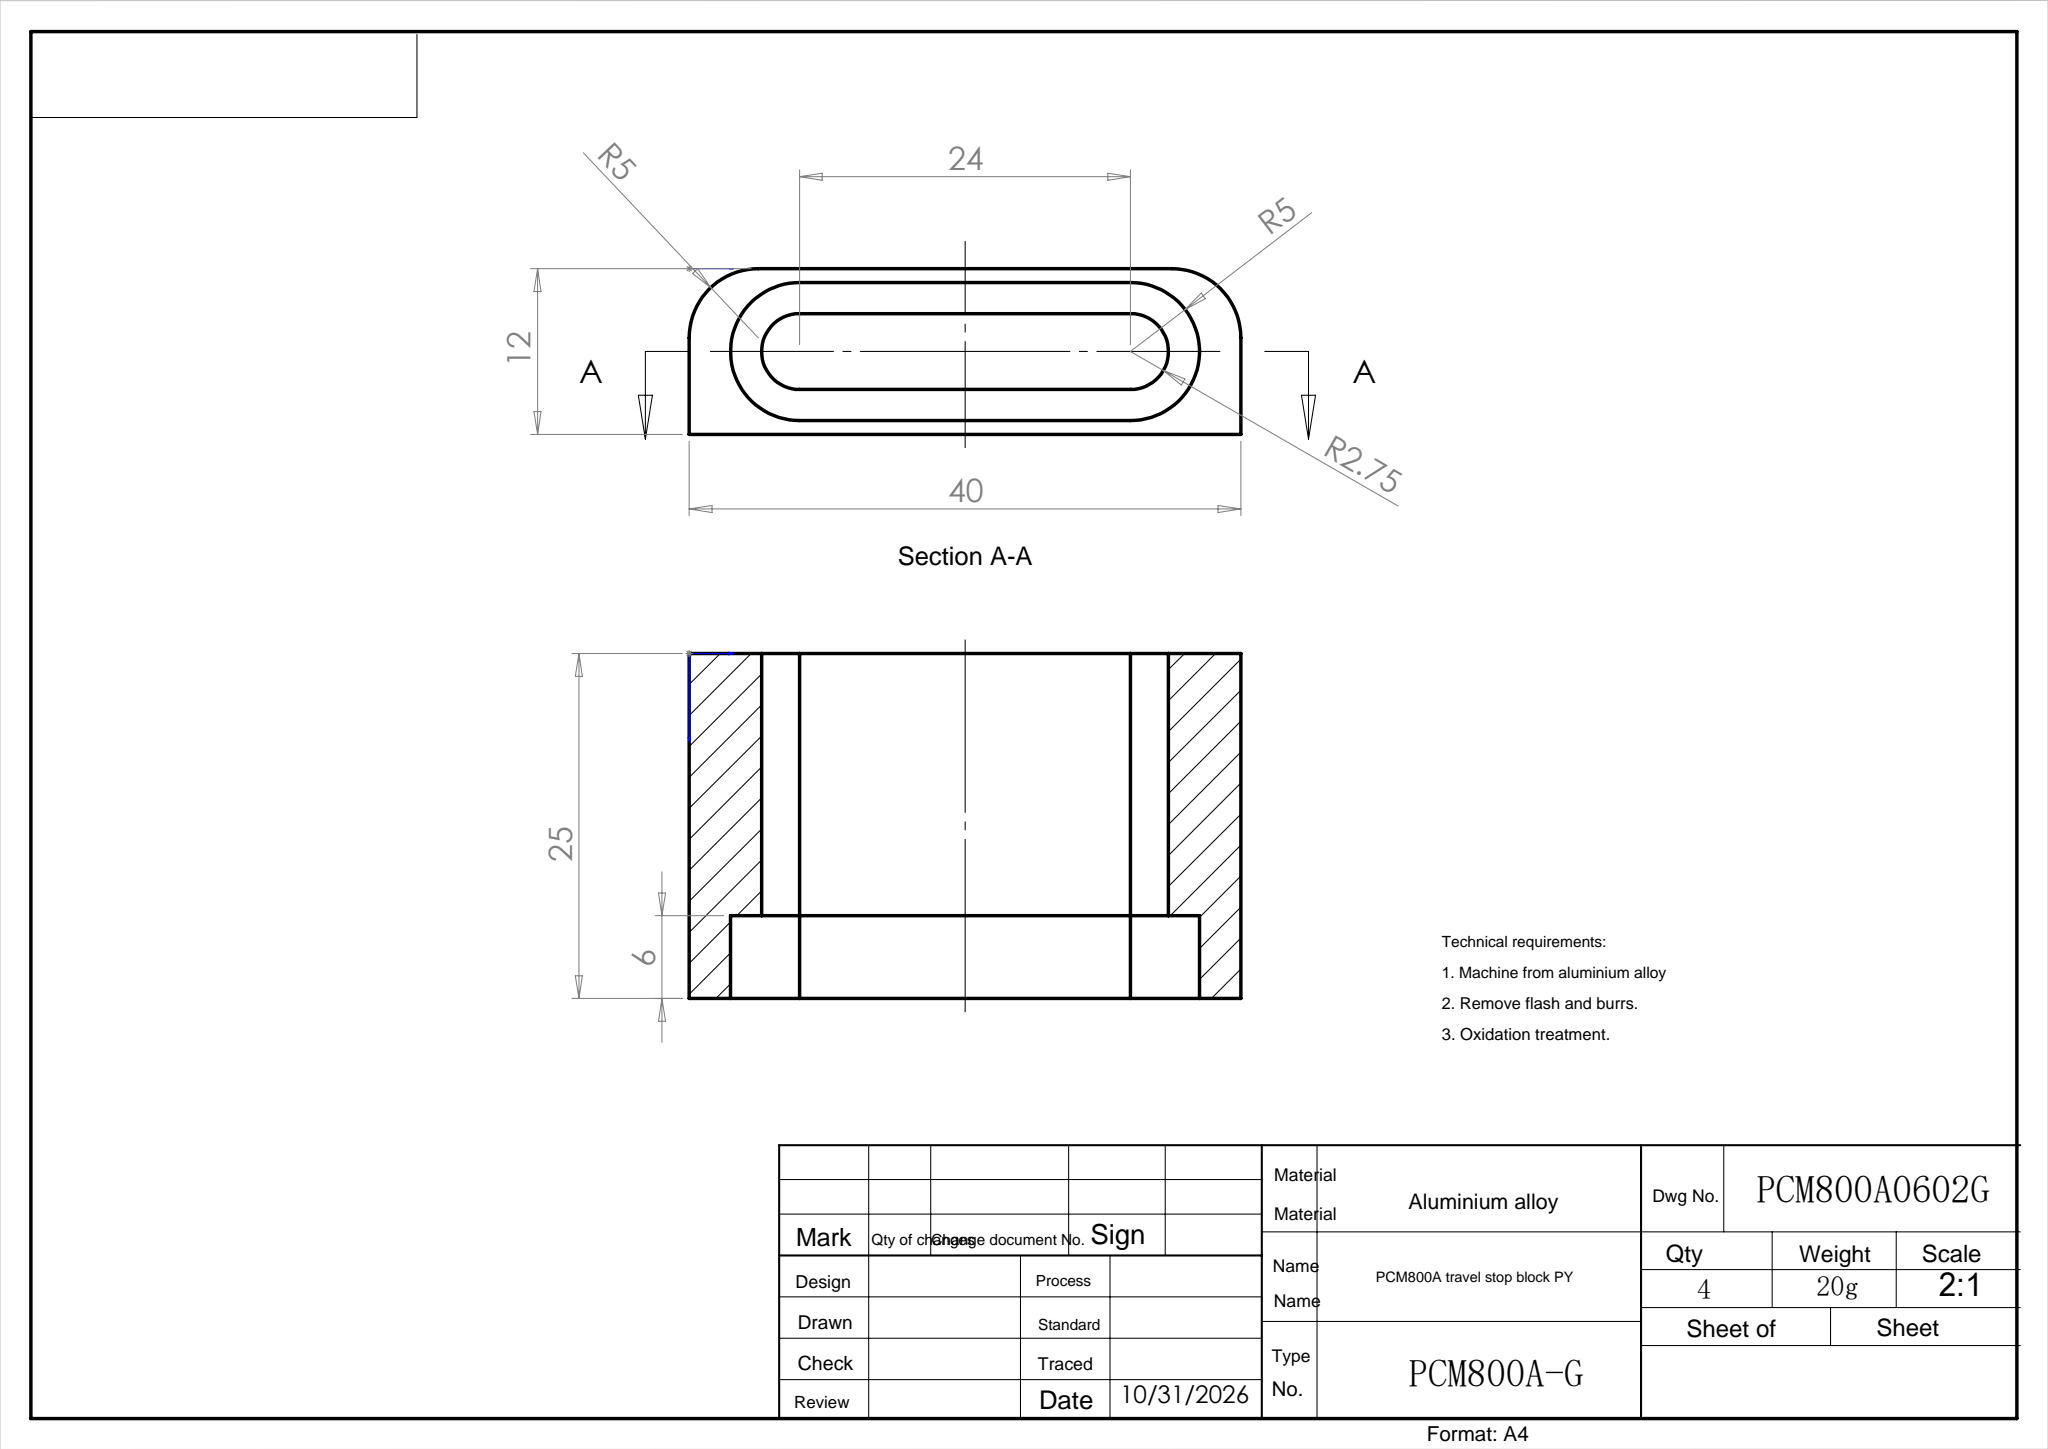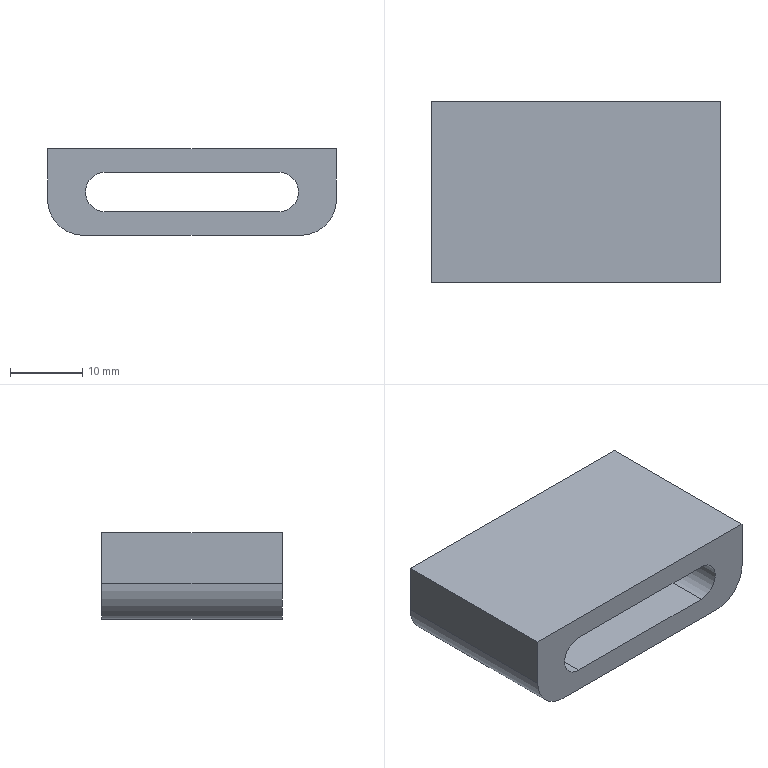Part | SolidWorks | features ICE 2, Extrusion 1, Fillet 1 | 1 solid | 17 faces | box 40 x 25 x 12 mm | volume 6861 mm3 | plane 11 | cylinder 6 | commonest cylinder face diameters 10 x4 5.5 x2
STEP:
#1=CARTESIAN_POINT('',(0.,25.,12.));
#2=VERTEX_POINT('',#1);
#3=CARTESIAN_POINT('',(0.,25.,5.));
#4=VERTEX_POINT('',#3);
#5=CARTESIAN_POINT('',(0.,25.,12.));
#6=DIRECTION('',(0.,0.,-1.));
#7=VECTOR('',#6,1000.);
#8=LINE('',#5,#7);
#9=EDGE_CURVE('',#2,#4,#8,.T.);
#10=ORIENTED_EDGE('',*,*,#9,.T.);
#11=CARTESIAN_POINT('',(0.,0.,5.));
#12=VERTEX_POINT('',#11);
#13=CARTESIAN_POINT('',(0.,0.,5.));
#14=DIRECTION('',(0.,-1.,0.));
#15=VECTOR('',#14,1000.);
#16=LINE('',#13,#15);
#17=EDGE_CURVE('',#4,#12,#16,.T.);
#18=ORIENTED_EDGE('',*,*,#17,.T.);
#19=CARTESIAN_POINT('',(0.,0.,12.));
#20=VERTEX_POINT('',#19);
#21=CARTESIAN_POINT('',(0.,0.,12.));
#22=DIRECTION('',(0.,0.,-1.));
#23=VECTOR('',#22,1000.);
#24=LINE('',#21,#23);
#25=EDGE_CURVE('',#20,#12,#24,.T.);
#26=ORIENTED_EDGE('',*,*,#25,.F.);
#27=CARTESIAN_POINT('',(0.,0.,12.));
#28=DIRECTION('',(0.,-1.,0.));
#29=VECTOR('',#28,1000.);
#30=LINE('',#27,#29);
#31=EDGE_CURVE('',#2,#20,#30,.T.);
#32=ORIENTED_EDGE('',*,*,#31,.F.);
#33=EDGE_LOOP('',(#10,#18,#26,#32));
#34=FACE_OUTER_BOUND('',#33,.T.);
#35=CARTESIAN_POINT('',(0.,0.,12.));
#36=DIRECTION('',(1.,0.,0.));
#37=DIRECTION('',(0.,0.,-1.));
#38=AXIS2_PLACEMENT_3D('',#35,#36,#37);
#39=PLANE('',#38);
#40=ADVANCED_FACE('',(#34),#39,.F.);
#41=CARTESIAN_POINT('',(32.,0.,3.25));
#42=VERTEX_POINT('',#41);
#43=CARTESIAN_POINT('',(8.,0.,3.25));
#44=VERTEX_POINT('',#43);
#45=CARTESIAN_POINT('',(32.,0.,3.25));
#46=DIRECTION('',(-1.,0.,0.));
#47=VECTOR('',#46,1000.);
#48=LINE('',#45,#47);
#49=EDGE_CURVE('',#42,#44,#48,.T.);
#50=ORIENTED_EDGE('',*,*,#49,.T.);
#51=CARTESIAN_POINT('',(8.,0.,8.75));
#52=VERTEX_POINT('',#51);
#53=CARTESIAN_POINT('',(8.,0.,6.));
#54=DIRECTION('',(0.,1.,0.));
#55=DIRECTION('',(0.,0.,1.));
#56=AXIS2_PLACEMENT_3D('',#53,#54,#55);
#57=CIRCLE('',#56,2.75);
#58=EDGE_CURVE('',#44,#52,#57,.T.);
#59=ORIENTED_EDGE('',*,*,#58,.T.);
#60=CARTESIAN_POINT('',(32.,0.,8.75));
#61=VERTEX_POINT('',#60);
#62=CARTESIAN_POINT('',(8.,0.,8.75));
#63=DIRECTION('',(1.,0.,0.));
#64=VECTOR('',#63,1000.);
#65=LINE('',#62,#64);
#66=EDGE_CURVE('',#52,#61,#65,.T.);
#67=ORIENTED_EDGE('',*,*,#66,.T.);
#68=CARTESIAN_POINT('',(32.,0.,6.));
#69=DIRECTION('',(0.,1.,0.));
#70=DIRECTION('',(0.,0.,1.));
#71=AXIS2_PLACEMENT_3D('',#68,#69,#70);
#72=CIRCLE('',#71,2.75);
#73=EDGE_CURVE('',#61,#42,#72,.T.);
#74=ORIENTED_EDGE('',*,*,#73,.T.);
#75=EDGE_LOOP('',(#50,#59,#67,#74));
#76=FACE_BOUND('',#75,.T.);
#77=ORIENTED_EDGE('',*,*,#25,.T.);
#78=CARTESIAN_POINT('',(5.,0.,0.));
#79=VERTEX_POINT('',#78);
#80=CARTESIAN_POINT('',(5.,0.,5.));
#81=DIRECTION('',(0.,-1.,0.));
#82=DIRECTION('',(0.,0.,1.));
#83=AXIS2_PLACEMENT_3D('',#80,#81,#82);
#84=CIRCLE('',#83,5.);
#85=EDGE_CURVE('',#12,#79,#84,.T.);
#86=ORIENTED_EDGE('',*,*,#85,.T.);
#87=CARTESIAN_POINT('',(35.,0.,0.));
#88=VERTEX_POINT('',#87);
#89=CARTESIAN_POINT('',(0.,0.,0.));
#90=DIRECTION('',(1.,0.,0.));
#91=VECTOR('',#90,1000.);
#92=LINE('',#89,#91);
#93=EDGE_CURVE('',#79,#88,#92,.T.);
#94=ORIENTED_EDGE('',*,*,#93,.T.);
#95=CARTESIAN_POINT('',(40.,0.,5.));
#96=VERTEX_POINT('',#95);
#97=CARTESIAN_POINT('',(35.,0.,5.));
#98=DIRECTION('',(0.,-1.,0.));
#99=DIRECTION('',(0.,0.,1.));
#100=AXIS2_PLACEMENT_3D('',#97,#98,#99);
#101=CIRCLE('',#100,5.);
#102=EDGE_CURVE('',#88,#96,#101,.T.);
#103=ORIENTED_EDGE('',*,*,#102,.T.);
#104=CARTESIAN_POINT('',(40.,0.,12.));
#105=VERTEX_POINT('',#104);
#106=CARTESIAN_POINT('',(40.,0.,12.));
#107=DIRECTION('',(0.,0.,-1.));
#108=VECTOR('',#107,1000.);
#109=LINE('',#106,#108);
#110=EDGE_CURVE('',#105,#96,#109,.T.);
#111=ORIENTED_EDGE('',*,*,#110,.F.);
#112=CARTESIAN_POINT('',(0.,0.,12.));
#113=DIRECTION('',(1.,0.,0.));
#114=VECTOR('',#113,1000.);
#115=LINE('',#112,#114);
#116=EDGE_CURVE('',#20,#105,#115,.T.);
#117=ORIENTED_EDGE('',*,*,#116,.F.);
#118=EDGE_LOOP('',(#77,#86,#94,#103,#111,#117));
#119=FACE_OUTER_BOUND('',#118,.T.);
#120=CARTESIAN_POINT('',(0.,0.,12.));
#121=DIRECTION('',(0.,1.,0.));
#122=DIRECTION('',(0.,0.,1.));
#123=AXIS2_PLACEMENT_3D('',#120,#121,#122);
#124=PLANE('',#123);
#125=ADVANCED_FACE('',(#76,#119),#124,.F.);
#126=ORIENTED_EDGE('',*,*,#110,.T.);
#127=CARTESIAN_POINT('',(40.,25.,5.));
#128=VERTEX_POINT('',#127);
#129=CARTESIAN_POINT('',(40.,25.,5.));
#130=DIRECTION('',(0.,1.,0.));
#131=VECTOR('',#130,1000.);
#132=LINE('',#129,#131);
#133=EDGE_CURVE('',#96,#128,#132,.T.);
#134=ORIENTED_EDGE('',*,*,#133,.T.);
#135=CARTESIAN_POINT('',(40.,25.,12.));
#136=VERTEX_POINT('',#135);
#137=CARTESIAN_POINT('',(40.,25.,12.));
#138=DIRECTION('',(0.,0.,-1.));
#139=VECTOR('',#138,1000.);
#140=LINE('',#137,#139);
#141=EDGE_CURVE('',#136,#128,#140,.T.);
#142=ORIENTED_EDGE('',*,*,#141,.F.);
#143=CARTESIAN_POINT('',(40.,0.,12.));
#144=DIRECTION('',(0.,1.,0.));
#145=VECTOR('',#144,1000.);
#146=LINE('',#143,#145);
#147=EDGE_CURVE('',#105,#136,#146,.T.);
#148=ORIENTED_EDGE('',*,*,#147,.F.);
#149=EDGE_LOOP('',(#126,#134,#142,#148));
#150=FACE_OUTER_BOUND('',#149,.T.);
#151=CARTESIAN_POINT('',(40.,0.,12.));
#152=DIRECTION('',(-1.,0.,0.));
#153=DIRECTION('',(0.,0.,1.));
#154=AXIS2_PLACEMENT_3D('',#151,#152,#153);
#155=PLANE('',#154);
#156=ADVANCED_FACE('',(#150),#155,.F.);
#157=CARTESIAN_POINT('',(8.,25.,11.));
#158=VERTEX_POINT('',#157);
#159=CARTESIAN_POINT('',(32.,25.,11.));
#160=VERTEX_POINT('',#159);
#161=CARTESIAN_POINT('',(8.,25.,11.));
#162=DIRECTION('',(1.,0.,0.));
#163=VECTOR('',#162,1000.);
#164=LINE('',#161,#163);
#165=EDGE_CURVE('',#158,#160,#164,.T.);
#166=ORIENTED_EDGE('',*,*,#165,.F.);
#167=CARTESIAN_POINT('',(8.,25.,1.));
#168=VERTEX_POINT('',#167);
#169=CARTESIAN_POINT('',(8.,25.,6.));
#170=DIRECTION('',(0.,1.,0.));
#171=DIRECTION('',(0.,0.,1.));
#172=AXIS2_PLACEMENT_3D('',#169,#170,#171);
#173=CIRCLE('',#172,5.);
#174=EDGE_CURVE('',#168,#158,#173,.T.);
#175=ORIENTED_EDGE('',*,*,#174,.F.);
#176=CARTESIAN_POINT('',(32.,25.,1.));
#177=VERTEX_POINT('',#176);
#178=CARTESIAN_POINT('',(8.,25.,1.));
#179=DIRECTION('',(-1.,0.,0.));
#180=VECTOR('',#179,1000.);
#181=LINE('',#178,#180);
#182=EDGE_CURVE('',#177,#168,#181,.T.);
#183=ORIENTED_EDGE('',*,*,#182,.F.);
#184=CARTESIAN_POINT('',(32.,25.,6.));
#185=DIRECTION('',(0.,1.,0.));
#186=DIRECTION('',(0.,0.,1.));
#187=AXIS2_PLACEMENT_3D('',#184,#185,#186);
#188=CIRCLE('',#187,5.);
#189=EDGE_CURVE('',#160,#177,#188,.T.);
#190=ORIENTED_EDGE('',*,*,#189,.F.);
#191=EDGE_LOOP('',(#166,#175,#183,#190));
#192=FACE_BOUND('',#191,.T.);
#193=CARTESIAN_POINT('',(35.,25.,0.));
#194=VERTEX_POINT('',#193);
#195=CARTESIAN_POINT('',(5.,25.,0.));
#196=VERTEX_POINT('',#195);
#197=CARTESIAN_POINT('',(0.,25.,0.));
#198=DIRECTION('',(-1.,0.,0.));
#199=VECTOR('',#198,1000.);
#200=LINE('',#197,#199);
#201=EDGE_CURVE('',#194,#196,#200,.T.);
#202=ORIENTED_EDGE('',*,*,#201,.T.);
#203=CARTESIAN_POINT('',(5.,25.,5.));
#204=DIRECTION('',(0.,1.,0.));
#205=DIRECTION('',(0.,0.,-1.));
#206=AXIS2_PLACEMENT_3D('',#203,#204,#205);
#207=CIRCLE('',#206,5.);
#208=EDGE_CURVE('',#196,#4,#207,.T.);
#209=ORIENTED_EDGE('',*,*,#208,.T.);
#210=ORIENTED_EDGE('',*,*,#9,.F.);
#211=CARTESIAN_POINT('',(0.,25.,12.));
#212=DIRECTION('',(-1.,0.,0.));
#213=VECTOR('',#212,1000.);
#214=LINE('',#211,#213);
#215=EDGE_CURVE('',#136,#2,#214,.T.);
#216=ORIENTED_EDGE('',*,*,#215,.F.);
#217=ORIENTED_EDGE('',*,*,#141,.T.);
#218=CARTESIAN_POINT('',(35.,25.,5.));
#219=DIRECTION('',(0.,1.,0.));
#220=DIRECTION('',(0.,0.,-1.));
#221=AXIS2_PLACEMENT_3D('',#218,#219,#220);
#222=CIRCLE('',#221,5.);
#223=EDGE_CURVE('',#128,#194,#222,.T.);
#224=ORIENTED_EDGE('',*,*,#223,.T.);
#225=EDGE_LOOP('',(#202,#209,#210,#216,#217,#224));
#226=FACE_OUTER_BOUND('',#225,.T.);
#227=CARTESIAN_POINT('',(0.,25.,12.));
#228=DIRECTION('',(0.,-1.,0.));
#229=DIRECTION('',(0.,0.,-1.));
#230=AXIS2_PLACEMENT_3D('',#227,#228,#229);
#231=PLANE('',#230);
#232=ADVANCED_FACE('',(#192,#226),#231,.F.);
#233=ORIENTED_EDGE('',*,*,#31,.T.);
#234=ORIENTED_EDGE('',*,*,#116,.T.);
#235=ORIENTED_EDGE('',*,*,#147,.T.);
#236=ORIENTED_EDGE('',*,*,#215,.T.);
#237=EDGE_LOOP('',(#233,#234,#235,#236));
#238=FACE_OUTER_BOUND('',#237,.T.);
#239=CARTESIAN_POINT('',(0.,25.,12.));
#240=DIRECTION('',(0.,0.,-1.));
#241=DIRECTION('',(-1.,0.,0.));
#242=AXIS2_PLACEMENT_3D('',#239,#240,#241);
#243=PLANE('',#242);
#244=ADVANCED_FACE('',(#238),#243,.F.);
#245=ORIENTED_EDGE('',*,*,#93,.F.);
#246=CARTESIAN_POINT('',(5.,25.,0.));
#247=DIRECTION('',(0.,1.,0.));
#248=VECTOR('',#247,1000.);
#249=LINE('',#246,#248);
#250=EDGE_CURVE('',#79,#196,#249,.T.);
#251=ORIENTED_EDGE('',*,*,#250,.T.);
#252=ORIENTED_EDGE('',*,*,#201,.F.);
#253=CARTESIAN_POINT('',(35.,0.,0.));
#254=DIRECTION('',(0.,-1.,0.));
#255=VECTOR('',#254,1000.);
#256=LINE('',#253,#255);
#257=EDGE_CURVE('',#194,#88,#256,.T.);
#258=ORIENTED_EDGE('',*,*,#257,.T.);
#259=EDGE_LOOP('',(#245,#251,#252,#258));
#260=FACE_OUTER_BOUND('',#259,.T.);
#261=CARTESIAN_POINT('',(0.,25.,0.));
#262=DIRECTION('',(0.,0.,-1.));
#263=DIRECTION('',(-1.,0.,0.));
#264=AXIS2_PLACEMENT_3D('',#261,#262,#263);
#265=PLANE('',#264);
#266=ADVANCED_FACE('',(#260),#265,.T.);
#267=ORIENTED_EDGE('',*,*,#174,.T.);
#268=CARTESIAN_POINT('',(8.,19.,11.));
#269=VERTEX_POINT('',#268);
#270=CARTESIAN_POINT('',(8.,19.,11.));
#271=DIRECTION('',(0.,1.,0.));
#272=VECTOR('',#271,1000.);
#273=LINE('',#270,#272);
#274=EDGE_CURVE('',#269,#158,#273,.T.);
#275=ORIENTED_EDGE('',*,*,#274,.F.);
#276=CARTESIAN_POINT('',(8.,19.,1.));
#277=VERTEX_POINT('',#276);
#278=CARTESIAN_POINT('',(8.,19.,6.));
#279=DIRECTION('',(0.,1.,0.));
#280=DIRECTION('',(0.,0.,1.));
#281=AXIS2_PLACEMENT_3D('',#278,#279,#280);
#282=CIRCLE('',#281,5.);
#283=EDGE_CURVE('',#277,#269,#282,.T.);
#284=ORIENTED_EDGE('',*,*,#283,.F.);
#285=CARTESIAN_POINT('',(8.,19.,1.));
#286=DIRECTION('',(0.,1.,0.));
#287=VECTOR('',#286,1000.);
#288=LINE('',#285,#287);
#289=EDGE_CURVE('',#277,#168,#288,.T.);
#290=ORIENTED_EDGE('',*,*,#289,.T.);
#291=EDGE_LOOP('',(#267,#275,#284,#290));
#292=FACE_OUTER_BOUND('',#291,.T.);
#293=CARTESIAN_POINT('',(8.,19.,6.));
#294=DIRECTION('',(0.,1.,0.));
#295=DIRECTION('',(0.,0.,1.));
#296=AXIS2_PLACEMENT_3D('',#293,#294,#295);
#297=CYLINDRICAL_SURFACE('',#296,5.);
#298=ADVANCED_FACE('',(#292),#297,.F.);
#299=ORIENTED_EDGE('',*,*,#182,.T.);
#300=ORIENTED_EDGE('',*,*,#289,.F.);
#301=CARTESIAN_POINT('',(32.,19.,1.));
#302=VERTEX_POINT('',#301);
#303=CARTESIAN_POINT('',(8.,19.,1.));
#304=DIRECTION('',(-1.,0.,0.));
#305=VECTOR('',#304,1000.);
#306=LINE('',#303,#305);
#307=EDGE_CURVE('',#302,#277,#306,.T.);
#308=ORIENTED_EDGE('',*,*,#307,.F.);
#309=CARTESIAN_POINT('',(32.,19.,1.));
#310=DIRECTION('',(0.,1.,0.));
#311=VECTOR('',#310,1000.);
#312=LINE('',#309,#311);
#313=EDGE_CURVE('',#302,#177,#312,.T.);
#314=ORIENTED_EDGE('',*,*,#313,.T.);
#315=EDGE_LOOP('',(#299,#300,#308,#314));
#316=FACE_OUTER_BOUND('',#315,.T.);
#317=CARTESIAN_POINT('',(8.,19.,1.));
#318=DIRECTION('',(0.,0.,-1.));
#319=DIRECTION('',(-1.,0.,0.));
#320=AXIS2_PLACEMENT_3D('',#317,#318,#319);
#321=PLANE('',#320);
#322=ADVANCED_FACE('',(#316),#321,.F.);
#323=ORIENTED_EDGE('',*,*,#189,.T.);
#324=ORIENTED_EDGE('',*,*,#313,.F.);
#325=CARTESIAN_POINT('',(32.,19.,11.));
#326=VERTEX_POINT('',#325);
#327=CARTESIAN_POINT('',(32.,19.,6.));
#328=DIRECTION('',(0.,1.,0.));
#329=DIRECTION('',(0.,0.,1.));
#330=AXIS2_PLACEMENT_3D('',#327,#328,#329);
#331=CIRCLE('',#330,5.);
#332=EDGE_CURVE('',#326,#302,#331,.T.);
#333=ORIENTED_EDGE('',*,*,#332,.F.);
#334=CARTESIAN_POINT('',(32.,19.,11.));
#335=DIRECTION('',(0.,1.,0.));
#336=VECTOR('',#335,1000.);
#337=LINE('',#334,#336);
#338=EDGE_CURVE('',#326,#160,#337,.T.);
#339=ORIENTED_EDGE('',*,*,#338,.T.);
#340=EDGE_LOOP('',(#323,#324,#333,#339));
#341=FACE_OUTER_BOUND('',#340,.T.);
#342=CARTESIAN_POINT('',(32.,19.,6.));
#343=DIRECTION('',(0.,1.,0.));
#344=DIRECTION('',(0.,0.,1.));
#345=AXIS2_PLACEMENT_3D('',#342,#343,#344);
#346=CYLINDRICAL_SURFACE('',#345,5.);
#347=ADVANCED_FACE('',(#341),#346,.F.);
#348=ORIENTED_EDGE('',*,*,#165,.T.);
#349=ORIENTED_EDGE('',*,*,#338,.F.);
#350=CARTESIAN_POINT('',(8.,19.,11.));
#351=DIRECTION('',(1.,0.,0.));
#352=VECTOR('',#351,1000.);
#353=LINE('',#350,#352);
#354=EDGE_CURVE('',#269,#326,#353,.T.);
#355=ORIENTED_EDGE('',*,*,#354,.F.);
#356=ORIENTED_EDGE('',*,*,#274,.T.);
#357=EDGE_LOOP('',(#348,#349,#355,#356));
#358=FACE_OUTER_BOUND('',#357,.T.);
#359=CARTESIAN_POINT('',(8.,19.,11.));
#360=DIRECTION('',(0.,0.,1.));
#361=DIRECTION('',(1.,0.,0.));
#362=AXIS2_PLACEMENT_3D('',#359,#360,#361);
#363=PLANE('',#362);
#364=ADVANCED_FACE('',(#358),#363,.F.);
#365=CARTESIAN_POINT('',(8.,19.,3.25));
#366=VERTEX_POINT('',#365);
#367=CARTESIAN_POINT('',(8.,19.,8.75));
#368=VERTEX_POINT('',#367);
#369=CARTESIAN_POINT('',(8.,19.,6.));
#370=DIRECTION('',(0.,1.,0.));
#371=DIRECTION('',(0.,0.,1.));
#372=AXIS2_PLACEMENT_3D('',#369,#370,#371);
#373=CIRCLE('',#372,2.75);
#374=EDGE_CURVE('',#366,#368,#373,.T.);
#375=ORIENTED_EDGE('',*,*,#374,.F.);
#376=CARTESIAN_POINT('',(32.,19.,3.25));
#377=VERTEX_POINT('',#376);
#378=CARTESIAN_POINT('',(32.,19.,3.25));
#379=DIRECTION('',(-1.,0.,0.));
#380=VECTOR('',#379,1000.);
#381=LINE('',#378,#380);
#382=EDGE_CURVE('',#377,#366,#381,.T.);
#383=ORIENTED_EDGE('',*,*,#382,.F.);
#384=CARTESIAN_POINT('',(32.,19.,8.75));
#385=VERTEX_POINT('',#384);
#386=CARTESIAN_POINT('',(32.,19.,6.));
#387=DIRECTION('',(0.,1.,0.));
#388=DIRECTION('',(0.,0.,1.));
#389=AXIS2_PLACEMENT_3D('',#386,#387,#388);
#390=CIRCLE('',#389,2.75);
#391=EDGE_CURVE('',#385,#377,#390,.T.);
#392=ORIENTED_EDGE('',*,*,#391,.F.);
#393=CARTESIAN_POINT('',(8.,19.,8.75));
#394=DIRECTION('',(1.,0.,0.));
#395=VECTOR('',#394,1000.);
#396=LINE('',#393,#395);
#397=EDGE_CURVE('',#368,#385,#396,.T.);
#398=ORIENTED_EDGE('',*,*,#397,.F.);
#399=EDGE_LOOP('',(#375,#383,#392,#398));
#400=FACE_BOUND('',#399,.T.);
#401=ORIENTED_EDGE('',*,*,#283,.T.);
#402=ORIENTED_EDGE('',*,*,#354,.T.);
#403=ORIENTED_EDGE('',*,*,#332,.T.);
#404=ORIENTED_EDGE('',*,*,#307,.T.);
#405=EDGE_LOOP('',(#401,#402,#403,#404));
#406=FACE_OUTER_BOUND('',#405,.T.);
#407=CARTESIAN_POINT('',(8.,19.,6.));
#408=DIRECTION('',(0.,1.,0.));
#409=DIRECTION('',(0.,0.,1.));
#410=AXIS2_PLACEMENT_3D('',#407,#408,#409);
#411=PLANE('',#410);
#412=ADVANCED_FACE('',(#400,#406),#411,.T.);
#413=ORIENTED_EDGE('',*,*,#374,.T.);
#414=CARTESIAN_POINT('',(8.,0.,8.75));
#415=DIRECTION('',(0.,1.,0.));
#416=VECTOR('',#415,1000.);
#417=LINE('',#414,#416);
#418=EDGE_CURVE('',#52,#368,#417,.T.);
#419=ORIENTED_EDGE('',*,*,#418,.F.);
#420=ORIENTED_EDGE('',*,*,#58,.F.);
#421=CARTESIAN_POINT('',(8.,0.,3.25));
#422=DIRECTION('',(0.,1.,0.));
#423=VECTOR('',#422,1000.);
#424=LINE('',#421,#423);
#425=EDGE_CURVE('',#44,#366,#424,.T.);
#426=ORIENTED_EDGE('',*,*,#425,.T.);
#427=EDGE_LOOP('',(#413,#419,#420,#426));
#428=FACE_OUTER_BOUND('',#427,.T.);
#429=CARTESIAN_POINT('',(8.,0.,6.));
#430=DIRECTION('',(0.,1.,0.));
#431=DIRECTION('',(0.,0.,1.));
#432=AXIS2_PLACEMENT_3D('',#429,#430,#431);
#433=CYLINDRICAL_SURFACE('',#432,2.75);
#434=ADVANCED_FACE('',(#428),#433,.F.);
#435=ORIENTED_EDGE('',*,*,#382,.T.);
#436=ORIENTED_EDGE('',*,*,#425,.F.);
#437=ORIENTED_EDGE('',*,*,#49,.F.);
#438=CARTESIAN_POINT('',(32.,0.,3.25));
#439=DIRECTION('',(0.,1.,0.));
#440=VECTOR('',#439,1000.);
#441=LINE('',#438,#440);
#442=EDGE_CURVE('',#42,#377,#441,.T.);
#443=ORIENTED_EDGE('',*,*,#442,.T.);
#444=EDGE_LOOP('',(#435,#436,#437,#443));
#445=FACE_OUTER_BOUND('',#444,.T.);
#446=CARTESIAN_POINT('',(32.,0.,3.25));
#447=DIRECTION('',(0.,0.,-1.));
#448=DIRECTION('',(-1.,0.,0.));
#449=AXIS2_PLACEMENT_3D('',#446,#447,#448);
#450=PLANE('',#449);
#451=ADVANCED_FACE('',(#445),#450,.F.);
#452=ORIENTED_EDGE('',*,*,#391,.T.);
#453=ORIENTED_EDGE('',*,*,#442,.F.);
#454=ORIENTED_EDGE('',*,*,#73,.F.);
#455=CARTESIAN_POINT('',(32.,0.,8.75));
#456=DIRECTION('',(0.,1.,0.));
#457=VECTOR('',#456,1000.);
#458=LINE('',#455,#457);
#459=EDGE_CURVE('',#61,#385,#458,.T.);
#460=ORIENTED_EDGE('',*,*,#459,.T.);
#461=EDGE_LOOP('',(#452,#453,#454,#460));
#462=FACE_OUTER_BOUND('',#461,.T.);
#463=CARTESIAN_POINT('',(32.,0.,6.));
#464=DIRECTION('',(0.,1.,0.));
#465=DIRECTION('',(0.,0.,1.));
#466=AXIS2_PLACEMENT_3D('',#463,#464,#465);
#467=CYLINDRICAL_SURFACE('',#466,2.75);
#468=ADVANCED_FACE('',(#462),#467,.F.);
#469=ORIENTED_EDGE('',*,*,#397,.T.);
#470=ORIENTED_EDGE('',*,*,#459,.F.);
#471=ORIENTED_EDGE('',*,*,#66,.F.);
#472=ORIENTED_EDGE('',*,*,#418,.T.);
#473=EDGE_LOOP('',(#469,#470,#471,#472));
#474=FACE_OUTER_BOUND('',#473,.T.);
#475=CARTESIAN_POINT('',(8.,0.,8.75));
#476=DIRECTION('',(0.,0.,1.));
#477=DIRECTION('',(1.,0.,0.));
#478=AXIS2_PLACEMENT_3D('',#475,#476,#477);
#479=PLANE('',#478);
#480=ADVANCED_FACE('',(#474),#479,.F.);
#481=ORIENTED_EDGE('',*,*,#208,.F.);
#482=ORIENTED_EDGE('',*,*,#250,.F.);
#483=ORIENTED_EDGE('',*,*,#85,.F.);
#484=ORIENTED_EDGE('',*,*,#17,.F.);
#485=EDGE_LOOP('',(#481,#482,#483,#484));
#486=FACE_OUTER_BOUND('',#485,.T.);
#487=CARTESIAN_POINT('',(5.,0.,5.));
#488=DIRECTION('',(0.,1.,0.));
#489=DIRECTION('',(0.,0.,1.));
#490=AXIS2_PLACEMENT_3D('',#487,#488,#489);
#491=CYLINDRICAL_SURFACE('',#490,5.);
#492=ADVANCED_FACE('',(#486),#491,.T.);
#493=ORIENTED_EDGE('',*,*,#102,.F.);
#494=ORIENTED_EDGE('',*,*,#257,.F.);
#495=ORIENTED_EDGE('',*,*,#223,.F.);
#496=ORIENTED_EDGE('',*,*,#133,.F.);
#497=EDGE_LOOP('',(#493,#494,#495,#496));
#498=FACE_OUTER_BOUND('',#497,.T.);
#499=CARTESIAN_POINT('',(35.,0.,5.));
#500=DIRECTION('',(0.,-1.,0.));
#501=DIRECTION('',(0.,0.,-1.));
#502=AXIS2_PLACEMENT_3D('',#499,#500,#501);
#503=CYLINDRICAL_SURFACE('',#502,5.);
#504=ADVANCED_FACE('',(#498),#503,.T.);
#505=CLOSED_SHELL('',(#40,#125,#156,#232,#244,#266,#298,#322,#347,#364,#412,#434,#451,#468,#480,#492,#504));
#506=MANIFOLD_SOLID_BREP('',#505);
#507=CARTESIAN_POINT('',(0.,0.,0.));
#508=DIRECTION('',(0.,0.,1.));
#509=DIRECTION('',(1.,0.,0.));
#510=AXIS2_PLACEMENT_3D('',#507,#508,#509);
#511=(LENGTH_UNIT()NAMED_UNIT(*)SI_UNIT(.MILLI.,.METRE.));
#512=UNCERTAINTY_MEASURE_WITH_UNIT(LENGTH_MEASURE(0.00001),#511,'','');
#513=(NAMED_UNIT(*)PLANE_ANGLE_UNIT()SI_UNIT($,.RADIAN.));
#514=(NAMED_UNIT(*)SI_UNIT($,.STERADIAN.)SOLID_ANGLE_UNIT());
#515=(GEOMETRIC_REPRESENTATION_CONTEXT(3)GLOBAL_UNCERTAINTY_ASSIGNED_CONTEXT((#512))GLOBAL_UNIT_ASSIGNED_CONTEXT((#511,#513,#514))REPRESENTATION_CONTEXT('',''));
#516=ADVANCED_BREP_SHAPE_REPRESENTATION('',(#506,#510),#515);